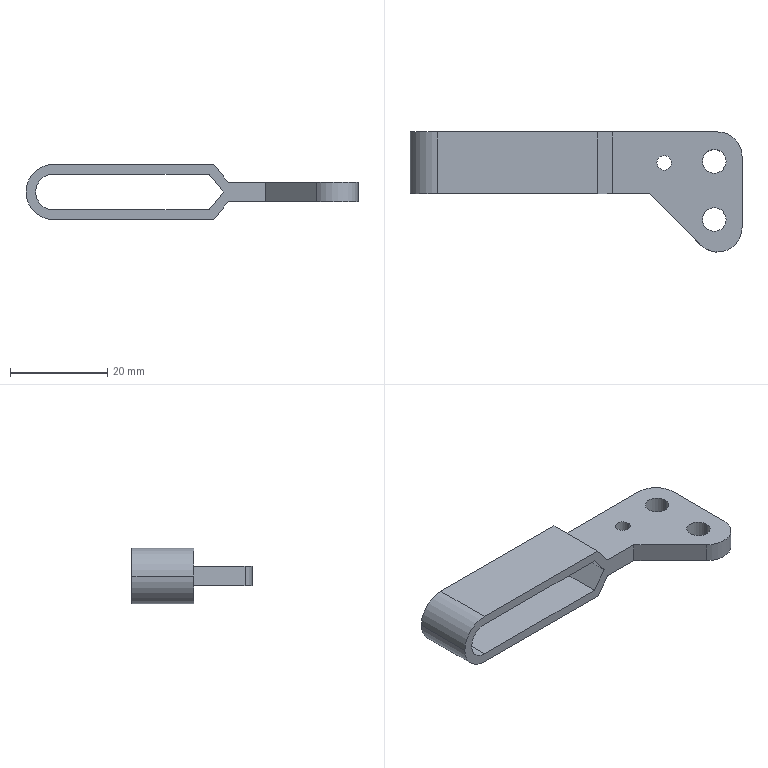Part | STEP file | 11-ARM_MC01-S311 | 1 solid | 25 faces | box 68.35 x 24.739 x 11.4 mm | volume 4057 mm3 | plane 14 | cylinder 11 | commonest cylinder face diameters 4.85 x4 3 x2 10 x2 11.4 x2 7.4 x1
STEP:
#1=CARTESIAN_POINT('',(-11.8,11.69,-4.));
#2=VERTEX_POINT('',#1);
#3=CARTESIAN_POINT('',(-8.8,11.69,-4.));
#4=VERTEX_POINT('',#3);
#5=CARTESIAN_POINT('',(-10.3,11.69,-4.));
#6=DIRECTION('',(0.,0.,1.));
#7=DIRECTION('',(1.,0.,0.));
#8=AXIS2_PLACEMENT_3D('',#5,#6,#7);
#9=CIRCLE('',#8,1.5);
#10=EDGE_CURVE('',#2,#4,#9,.T.);
#11=ORIENTED_EDGE('',*,*,#10,.F.);
#12=CARTESIAN_POINT('',(-11.8,11.69,0.));
#13=VERTEX_POINT('',#12);
#14=CARTESIAN_POINT('',(-11.8,11.69,0.));
#15=DIRECTION('',(0.,0.,1.));
#16=VECTOR('',#15,1000.);
#17=LINE('',#14,#16);
#18=EDGE_CURVE('',#2,#13,#17,.T.);
#19=ORIENTED_EDGE('',*,*,#18,.T.);
#20=CARTESIAN_POINT('',(-8.8,11.69,0.));
#21=VERTEX_POINT('',#20);
#22=CARTESIAN_POINT('',(-10.3,11.69,0.));
#23=DIRECTION('',(0.,0.,1.));
#24=DIRECTION('',(1.,0.,0.));
#25=AXIS2_PLACEMENT_3D('',#22,#23,#24);
#26=CIRCLE('',#25,1.5);
#27=EDGE_CURVE('',#13,#21,#26,.T.);
#28=ORIENTED_EDGE('',*,*,#27,.T.);
#29=CARTESIAN_POINT('',(-8.8,11.69,0.));
#30=DIRECTION('',(0.,0.,1.));
#31=VECTOR('',#30,1000.);
#32=LINE('',#29,#31);
#33=EDGE_CURVE('',#4,#21,#32,.T.);
#34=ORIENTED_EDGE('',*,*,#33,.F.);
#35=EDGE_LOOP('',(#11,#19,#28,#34));
#36=FACE_OUTER_BOUND('',#35,.T.);
#37=CARTESIAN_POINT('',(-10.3,11.69,0.));
#38=DIRECTION('',(0.,0.,1.));
#39=DIRECTION('',(1.,0.,0.));
#40=AXIS2_PLACEMENT_3D('',#37,#38,#39);
#41=CYLINDRICAL_SURFACE('',#40,1.5);
#42=ADVANCED_FACE('',(#36),#41,.F.);
#43=CARTESIAN_POINT('',(-2.425,12.,-4.));
#44=VERTEX_POINT('',#43);
#45=CARTESIAN_POINT('',(2.425,12.,-4.));
#46=VERTEX_POINT('',#45);
#47=CARTESIAN_POINT('',(0.,12.,-4.));
#48=DIRECTION('',(0.,0.,1.));
#49=DIRECTION('',(1.,0.,0.));
#50=AXIS2_PLACEMENT_3D('',#47,#48,#49);
#51=CIRCLE('',#50,2.425);
#52=EDGE_CURVE('',#44,#46,#51,.T.);
#53=ORIENTED_EDGE('',*,*,#52,.F.);
#54=CARTESIAN_POINT('',(-2.425,12.,0.));
#55=VERTEX_POINT('',#54);
#56=CARTESIAN_POINT('',(-2.425,12.,0.));
#57=DIRECTION('',(0.,0.,1.));
#58=VECTOR('',#57,1000.);
#59=LINE('',#56,#58);
#60=EDGE_CURVE('',#44,#55,#59,.T.);
#61=ORIENTED_EDGE('',*,*,#60,.T.);
#62=CARTESIAN_POINT('',(2.425,12.,0.));
#63=VERTEX_POINT('',#62);
#64=CARTESIAN_POINT('',(0.,12.,0.));
#65=DIRECTION('',(0.,0.,1.));
#66=DIRECTION('',(1.,0.,0.));
#67=AXIS2_PLACEMENT_3D('',#64,#65,#66);
#68=CIRCLE('',#67,2.425);
#69=EDGE_CURVE('',#55,#63,#68,.T.);
#70=ORIENTED_EDGE('',*,*,#69,.T.);
#71=CARTESIAN_POINT('',(2.425,12.,0.));
#72=DIRECTION('',(0.,0.,1.));
#73=VECTOR('',#72,1000.);
#74=LINE('',#71,#73);
#75=EDGE_CURVE('',#46,#63,#74,.T.);
#76=ORIENTED_EDGE('',*,*,#75,.F.);
#77=EDGE_LOOP('',(#53,#61,#70,#76));
#78=FACE_OUTER_BOUND('',#77,.T.);
#79=CARTESIAN_POINT('',(0.,12.,0.));
#80=DIRECTION('',(0.,0.,1.));
#81=DIRECTION('',(1.,0.,0.));
#82=AXIS2_PLACEMENT_3D('',#79,#80,#81);
#83=CYLINDRICAL_SURFACE('',#82,2.425);
#84=ADVANCED_FACE('',(#78),#83,.F.);
#85=CARTESIAN_POINT('',(-2.425,0.,-4.));
#86=VERTEX_POINT('',#85);
#87=CARTESIAN_POINT('',(2.425,0.,-4.));
#88=VERTEX_POINT('',#87);
#89=CARTESIAN_POINT('',(0.,0.,-4.));
#90=DIRECTION('',(0.,0.,1.));
#91=DIRECTION('',(1.,0.,0.));
#92=AXIS2_PLACEMENT_3D('',#89,#90,#91);
#93=CIRCLE('',#92,2.425);
#94=EDGE_CURVE('',#86,#88,#93,.T.);
#95=ORIENTED_EDGE('',*,*,#94,.F.);
#96=CARTESIAN_POINT('',(-2.425,0.,0.));
#97=VERTEX_POINT('',#96);
#98=CARTESIAN_POINT('',(-2.425,0.,0.));
#99=DIRECTION('',(0.,0.,1.));
#100=VECTOR('',#99,1000.);
#101=LINE('',#98,#100);
#102=EDGE_CURVE('',#86,#97,#101,.T.);
#103=ORIENTED_EDGE('',*,*,#102,.T.);
#104=CARTESIAN_POINT('',(2.425,0.,0.));
#105=VERTEX_POINT('',#104);
#106=CARTESIAN_POINT('',(0.,0.,0.));
#107=DIRECTION('',(0.,0.,1.));
#108=DIRECTION('',(1.,0.,0.));
#109=AXIS2_PLACEMENT_3D('',#106,#107,#108);
#110=CIRCLE('',#109,2.425);
#111=EDGE_CURVE('',#97,#105,#110,.T.);
#112=ORIENTED_EDGE('',*,*,#111,.T.);
#113=CARTESIAN_POINT('',(2.425,0.,0.));
#114=DIRECTION('',(0.,0.,1.));
#115=VECTOR('',#114,1000.);
#116=LINE('',#113,#115);
#117=EDGE_CURVE('',#88,#105,#116,.T.);
#118=ORIENTED_EDGE('',*,*,#117,.F.);
#119=EDGE_LOOP('',(#95,#103,#112,#118));
#120=FACE_OUTER_BOUND('',#119,.T.);
#121=CARTESIAN_POINT('',(0.,0.,0.));
#122=DIRECTION('',(0.,0.,1.));
#123=DIRECTION('',(1.,0.,0.));
#124=AXIS2_PLACEMENT_3D('',#121,#122,#123);
#125=CYLINDRICAL_SURFACE('',#124,2.425);
#126=ADVANCED_FACE('',(#120),#125,.F.);
#127=CARTESIAN_POINT('',(-21.998,18.05,-2.));
#128=VERTEX_POINT('',#127);
#129=CARTESIAN_POINT('',(-24.95,18.05,-5.7));
#130=VERTEX_POINT('',#129);
#131=CARTESIAN_POINT('',(-24.95,18.05,-5.7));
#132=DIRECTION('',(-0.6237,0.,-0.7817));
#133=VECTOR('',#132,1000.);
#134=LINE('',#131,#133);
#135=EDGE_CURVE('',#128,#130,#134,.T.);
#136=ORIENTED_EDGE('',*,*,#135,.F.);
#137=CARTESIAN_POINT('',(-24.95,18.05,1.7));
#138=VERTEX_POINT('',#137);
#139=CARTESIAN_POINT('',(-24.95,18.05,1.7));
#140=DIRECTION('',(0.6237,0.,-0.7817));
#141=VECTOR('',#140,1000.);
#142=LINE('',#139,#141);
#143=EDGE_CURVE('',#138,#128,#142,.T.);
#144=ORIENTED_EDGE('',*,*,#143,.F.);
#145=CARTESIAN_POINT('',(-56.95,18.05,1.7));
#146=VERTEX_POINT('',#145);
#147=CARTESIAN_POINT('',(-56.95,18.05,1.7));
#148=DIRECTION('',(1.,0.,0.));
#149=VECTOR('',#148,1000.);
#150=LINE('',#147,#149);
#151=EDGE_CURVE('',#146,#138,#150,.T.);
#152=ORIENTED_EDGE('',*,*,#151,.F.);
#153=CARTESIAN_POINT('',(-56.95,18.05,-5.7));
#154=VERTEX_POINT('',#153);
#155=CARTESIAN_POINT('',(-56.95,18.05,-2.));
#156=DIRECTION('',(0.,1.,0.));
#157=DIRECTION('',(0.,0.,1.));
#158=AXIS2_PLACEMENT_3D('',#155,#156,#157);
#159=CIRCLE('',#158,3.7);
#160=EDGE_CURVE('',#154,#146,#159,.T.);
#161=ORIENTED_EDGE('',*,*,#160,.F.);
#162=CARTESIAN_POINT('',(-24.95,18.05,-5.7));
#163=DIRECTION('',(-1.,0.,0.));
#164=VECTOR('',#163,1000.);
#165=LINE('',#162,#164);
#166=EDGE_CURVE('',#130,#154,#165,.T.);
#167=ORIENTED_EDGE('',*,*,#166,.F.);
#168=EDGE_LOOP('',(#136,#144,#152,#161,#167));
#169=FACE_BOUND('',#168,.T.);
#170=CARTESIAN_POINT('',(0.7,18.05,0.));
#171=VERTEX_POINT('',#170);
#172=CARTESIAN_POINT('',(-21.035,18.05,0.));
#173=VERTEX_POINT('',#172);
#174=CARTESIAN_POINT('',(-21.035,18.05,0.));
#175=DIRECTION('',(-1.,0.,0.));
#176=VECTOR('',#175,1000.);
#177=LINE('',#174,#176);
#178=EDGE_CURVE('',#171,#173,#177,.T.);
#179=ORIENTED_EDGE('',*,*,#178,.F.);
#180=CARTESIAN_POINT('',(0.7,18.05,-4.));
#181=VERTEX_POINT('',#180);
#182=CARTESIAN_POINT('',(0.7,18.05,3.7));
#183=DIRECTION('',(0.,0.,-1.));
#184=VECTOR('',#183,1000.);
#185=LINE('',#182,#184);
#186=EDGE_CURVE('',#171,#181,#185,.T.);
#187=ORIENTED_EDGE('',*,*,#186,.T.);
#188=CARTESIAN_POINT('',(-21.035,18.05,-4.));
#189=VERTEX_POINT('',#188);
#190=CARTESIAN_POINT('',(-21.035,18.05,-4.));
#191=DIRECTION('',(1.,0.,0.));
#192=VECTOR('',#191,1000.);
#193=LINE('',#190,#192);
#194=EDGE_CURVE('',#189,#181,#193,.T.);
#195=ORIENTED_EDGE('',*,*,#194,.F.);
#196=CARTESIAN_POINT('',(-23.987,18.05,-7.7));
#197=VERTEX_POINT('',#196);
#198=CARTESIAN_POINT('',(-23.987,18.05,-7.7));
#199=DIRECTION('',(0.6237,0.,0.7817));
#200=VECTOR('',#199,1000.);
#201=LINE('',#198,#200);
#202=EDGE_CURVE('',#197,#189,#201,.T.);
#203=ORIENTED_EDGE('',*,*,#202,.F.);
#204=CARTESIAN_POINT('',(-56.95,18.05,-7.7));
#205=VERTEX_POINT('',#204);
#206=CARTESIAN_POINT('',(-62.65,18.05,-7.7));
#207=DIRECTION('',(-1.,0.,0.));
#208=VECTOR('',#207,1000.);
#209=LINE('',#206,#208);
#210=EDGE_CURVE('',#197,#205,#209,.T.);
#211=ORIENTED_EDGE('',*,*,#210,.T.);
#212=CARTESIAN_POINT('',(-62.65,18.05,-2.));
#213=VERTEX_POINT('',#212);
#214=CARTESIAN_POINT('',(-56.95,18.05,-2.));
#215=DIRECTION('',(0.,1.,0.));
#216=DIRECTION('',(0.,0.,-1.));
#217=AXIS2_PLACEMENT_3D('',#214,#215,#216);
#218=CIRCLE('',#217,5.7);
#219=EDGE_CURVE('',#205,#213,#218,.T.);
#220=ORIENTED_EDGE('',*,*,#219,.T.);
#221=CARTESIAN_POINT('',(-56.95,18.05,3.7));
#222=VERTEX_POINT('',#221);
#223=CARTESIAN_POINT('',(-56.95,18.05,-2.));
#224=DIRECTION('',(0.,1.,0.));
#225=DIRECTION('',(0.,0.,-1.));
#226=AXIS2_PLACEMENT_3D('',#223,#224,#225);
#227=CIRCLE('',#226,5.7);
#228=EDGE_CURVE('',#213,#222,#227,.T.);
#229=ORIENTED_EDGE('',*,*,#228,.T.);
#230=CARTESIAN_POINT('',(-23.987,18.05,3.7));
#231=VERTEX_POINT('',#230);
#232=CARTESIAN_POINT('',(-62.65,18.05,3.7));
#233=DIRECTION('',(-1.,0.,0.));
#234=VECTOR('',#233,1000.);
#235=LINE('',#232,#234);
#236=EDGE_CURVE('',#231,#222,#235,.T.);
#237=ORIENTED_EDGE('',*,*,#236,.F.);
#238=CARTESIAN_POINT('',(-23.987,18.05,3.7));
#239=DIRECTION('',(-0.6237,0.,0.7817));
#240=VECTOR('',#239,1000.);
#241=LINE('',#238,#240);
#242=EDGE_CURVE('',#173,#231,#241,.T.);
#243=ORIENTED_EDGE('',*,*,#242,.F.);
#244=EDGE_LOOP('',(#179,#187,#195,#203,#211,#220,#229,#237,#243));
#245=FACE_OUTER_BOUND('',#244,.T.);
#246=CARTESIAN_POINT('',(-62.65,18.05,3.7));
#247=DIRECTION('',(0.,-1.,0.));
#248=DIRECTION('',(0.,0.,-1.));
#249=AXIS2_PLACEMENT_3D('',#246,#247,#248);
#250=PLANE('',#249);
#251=ADVANCED_FACE('',(#169,#245),#250,.F.);
#252=CARTESIAN_POINT('',(-56.95,5.35,1.7));
#253=VERTEX_POINT('',#252);
#254=CARTESIAN_POINT('',(-24.95,5.35,1.7));
#255=VERTEX_POINT('',#254);
#256=CARTESIAN_POINT('',(-62.65,5.35,1.7));
#257=DIRECTION('',(1.,0.,0.));
#258=VECTOR('',#257,1000.);
#259=LINE('',#256,#258);
#260=EDGE_CURVE('',#253,#255,#259,.T.);
#261=ORIENTED_EDGE('',*,*,#260,.T.);
#262=CARTESIAN_POINT('',(-21.998,5.35,-2.));
#263=VERTEX_POINT('',#262);
#264=CARTESIAN_POINT('',(-40.59,5.35,21.302));
#265=DIRECTION('',(0.6237,0.,-0.7817));
#266=VECTOR('',#265,1000.);
#267=LINE('',#264,#266);
#268=EDGE_CURVE('',#255,#263,#267,.T.);
#269=ORIENTED_EDGE('',*,*,#268,.T.);
#270=CARTESIAN_POINT('',(-24.95,5.35,-5.7));
#271=VERTEX_POINT('',#270);
#272=CARTESIAN_POINT('',(-35.032,5.35,-18.336));
#273=DIRECTION('',(-0.6237,0.,-0.7817));
#274=VECTOR('',#273,1000.);
#275=LINE('',#272,#274);
#276=EDGE_CURVE('',#263,#271,#275,.T.);
#277=ORIENTED_EDGE('',*,*,#276,.T.);
#278=CARTESIAN_POINT('',(-56.95,5.35,-5.7));
#279=VERTEX_POINT('',#278);
#280=CARTESIAN_POINT('',(-62.65,5.35,-5.7));
#281=DIRECTION('',(-1.,0.,0.));
#282=VECTOR('',#281,1000.);
#283=LINE('',#280,#282);
#284=EDGE_CURVE('',#271,#279,#283,.T.);
#285=ORIENTED_EDGE('',*,*,#284,.T.);
#286=CARTESIAN_POINT('',(-56.95,5.35,-2.));
#287=DIRECTION('',(0.,1.,0.));
#288=DIRECTION('',(-1.,0.,0.));
#289=AXIS2_PLACEMENT_3D('',#286,#287,#288);
#290=CIRCLE('',#289,3.7);
#291=EDGE_CURVE('',#279,#253,#290,.T.);
#292=ORIENTED_EDGE('',*,*,#291,.T.);
#293=EDGE_LOOP('',(#261,#269,#277,#285,#292));
#294=FACE_BOUND('',#293,.T.);
#295=CARTESIAN_POINT('',(-56.95,5.35,-7.7));
#296=VERTEX_POINT('',#295);
#297=CARTESIAN_POINT('',(-23.987,5.35,-7.7));
#298=VERTEX_POINT('',#297);
#299=CARTESIAN_POINT('',(-62.65,5.35,-7.7));
#300=DIRECTION('',(1.,0.,0.));
#301=VECTOR('',#300,1000.);
#302=LINE('',#299,#301);
#303=EDGE_CURVE('',#296,#298,#302,.T.);
#304=ORIENTED_EDGE('',*,*,#303,.T.);
#305=CARTESIAN_POINT('',(-21.035,5.35,-4.));
#306=VERTEX_POINT('',#305);
#307=CARTESIAN_POINT('',(-33.469,5.35,-19.583));
#308=DIRECTION('',(0.6237,0.,0.7817));
#309=VECTOR('',#308,1000.);
#310=LINE('',#307,#309);
#311=EDGE_CURVE('',#298,#306,#310,.T.);
#312=ORIENTED_EDGE('',*,*,#311,.T.);
#313=CARTESIAN_POINT('',(-13.41,5.35,-4.));
#314=VERTEX_POINT('',#313);
#315=CARTESIAN_POINT('',(-62.65,5.35,-4.));
#316=DIRECTION('',(1.,0.,0.));
#317=VECTOR('',#316,1000.);
#318=LINE('',#315,#317);
#319=EDGE_CURVE('',#306,#314,#318,.T.);
#320=ORIENTED_EDGE('',*,*,#319,.T.);
#321=CARTESIAN_POINT('',(-13.41,5.35,0.));
#322=VERTEX_POINT('',#321);
#323=CARTESIAN_POINT('',(-13.41,5.35,3.7));
#324=DIRECTION('',(0.,0.,-1.));
#325=VECTOR('',#324,1000.);
#326=LINE('',#323,#325);
#327=EDGE_CURVE('',#322,#314,#326,.T.);
#328=ORIENTED_EDGE('',*,*,#327,.F.);
#329=CARTESIAN_POINT('',(-21.035,5.35,0.));
#330=VERTEX_POINT('',#329);
#331=CARTESIAN_POINT('',(-62.65,5.35,0.));
#332=DIRECTION('',(-1.,0.,0.));
#333=VECTOR('',#332,1000.);
#334=LINE('',#331,#333);
#335=EDGE_CURVE('',#322,#330,#334,.T.);
#336=ORIENTED_EDGE('',*,*,#335,.T.);
#337=CARTESIAN_POINT('',(-23.987,5.35,3.7));
#338=VERTEX_POINT('',#337);
#339=CARTESIAN_POINT('',(-39.026,5.35,22.549));
#340=DIRECTION('',(-0.6237,0.,0.7817));
#341=VECTOR('',#340,1000.);
#342=LINE('',#339,#341);
#343=EDGE_CURVE('',#330,#338,#342,.T.);
#344=ORIENTED_EDGE('',*,*,#343,.T.);
#345=CARTESIAN_POINT('',(-56.95,5.35,3.7));
#346=VERTEX_POINT('',#345);
#347=CARTESIAN_POINT('',(-62.65,5.35,3.7));
#348=DIRECTION('',(1.,0.,0.));
#349=VECTOR('',#348,1000.);
#350=LINE('',#347,#349);
#351=EDGE_CURVE('',#346,#338,#350,.T.);
#352=ORIENTED_EDGE('',*,*,#351,.F.);
#353=CARTESIAN_POINT('',(-62.65,5.35,-2.));
#354=VERTEX_POINT('',#353);
#355=CARTESIAN_POINT('',(-56.95,5.35,-2.));
#356=DIRECTION('',(0.,-1.,0.));
#357=DIRECTION('',(-1.,0.,0.));
#358=AXIS2_PLACEMENT_3D('',#355,#356,#357);
#359=CIRCLE('',#358,5.7);
#360=EDGE_CURVE('',#346,#354,#359,.T.);
#361=ORIENTED_EDGE('',*,*,#360,.T.);
#362=CARTESIAN_POINT('',(-56.95,5.35,-2.));
#363=DIRECTION('',(0.,-1.,0.));
#364=DIRECTION('',(-1.,0.,0.));
#365=AXIS2_PLACEMENT_3D('',#362,#363,#364);
#366=CIRCLE('',#365,5.7);
#367=EDGE_CURVE('',#354,#296,#366,.T.);
#368=ORIENTED_EDGE('',*,*,#367,.T.);
#369=EDGE_LOOP('',(#304,#312,#320,#328,#336,#344,#352,#361,#368));
#370=FACE_OUTER_BOUND('',#369,.T.);
#371=CARTESIAN_POINT('',(-62.65,5.35,3.7));
#372=DIRECTION('',(0.,1.,0.));
#373=DIRECTION('',(-1.,0.,0.));
#374=AXIS2_PLACEMENT_3D('',#371,#372,#373);
#375=PLANE('',#374);
#376=ADVANCED_FACE('',(#294,#370),#375,.F.);
#377=ORIENTED_EDGE('',*,*,#327,.T.);
#378=CARTESIAN_POINT('',(-2.836,-5.224,-4.));
#379=VERTEX_POINT('',#378);
#380=CARTESIAN_POINT('',(-13.41,5.35,-4.));
#381=DIRECTION('',(0.7071,-0.7071,0.));
#382=VECTOR('',#381,1000.);
#383=LINE('',#380,#382);
#384=EDGE_CURVE('',#314,#379,#383,.T.);
#385=ORIENTED_EDGE('',*,*,#384,.T.);
#386=CARTESIAN_POINT('',(-2.836,-5.224,0.));
#387=VERTEX_POINT('',#386);
#388=CARTESIAN_POINT('',(-2.836,-5.224,3.7));
#389=DIRECTION('',(0.,0.,-1.));
#390=VECTOR('',#389,1000.);
#391=LINE('',#388,#390);
#392=EDGE_CURVE('',#387,#379,#391,.T.);
#393=ORIENTED_EDGE('',*,*,#392,.F.);
#394=CARTESIAN_POINT('',(-13.41,5.35,0.));
#395=DIRECTION('',(-0.7071,0.7071,0.));
#396=VECTOR('',#395,1000.);
#397=LINE('',#394,#396);
#398=EDGE_CURVE('',#387,#322,#397,.T.);
#399=ORIENTED_EDGE('',*,*,#398,.T.);
#400=EDGE_LOOP('',(#377,#385,#393,#399));
#401=FACE_OUTER_BOUND('',#400,.T.);
#402=CARTESIAN_POINT('',(-13.41,5.35,3.7));
#403=DIRECTION('',(0.7071,0.7071,0.));
#404=DIRECTION('',(-0.7071,0.7071,0.));
#405=AXIS2_PLACEMENT_3D('',#402,#403,#404);
#406=PLANE('',#405);
#407=ADVANCED_FACE('',(#401),#406,.F.);
#408=ORIENTED_EDGE('',*,*,#392,.T.);
#409=CARTESIAN_POINT('',(5.7,-1.689,-4.));
#410=VERTEX_POINT('',#409);
#411=CARTESIAN_POINT('',(0.7,-1.689,-4.));
#412=DIRECTION('',(0.,0.,1.));
#413=DIRECTION('',(1.,0.,0.));
#414=AXIS2_PLACEMENT_3D('',#411,#412,#413);
#415=CIRCLE('',#414,5.);
#416=EDGE_CURVE('',#379,#410,#415,.T.);
#417=ORIENTED_EDGE('',*,*,#416,.T.);
#418=CARTESIAN_POINT('',(5.7,-1.689,0.));
#419=VERTEX_POINT('',#418);
#420=CARTESIAN_POINT('',(5.7,-1.689,3.7));
#421=DIRECTION('',(0.,0.,-1.));
#422=VECTOR('',#421,1000.);
#423=LINE('',#420,#422);
#424=EDGE_CURVE('',#419,#410,#423,.T.);
#425=ORIENTED_EDGE('',*,*,#424,.F.);
#426=CARTESIAN_POINT('',(0.7,-1.689,0.));
#427=DIRECTION('',(0.,0.,-1.));
#428=DIRECTION('',(-1.,0.,0.));
#429=AXIS2_PLACEMENT_3D('',#426,#427,#428);
#430=CIRCLE('',#429,5.);
#431=EDGE_CURVE('',#419,#387,#430,.T.);
#432=ORIENTED_EDGE('',*,*,#431,.T.);
#433=EDGE_LOOP('',(#408,#417,#425,#432));
#434=FACE_OUTER_BOUND('',#433,.T.);
#435=CARTESIAN_POINT('',(0.7,-1.689,3.7));
#436=DIRECTION('',(0.,0.,-1.));
#437=DIRECTION('',(-1.,0.,0.));
#438=AXIS2_PLACEMENT_3D('',#435,#436,#437);
#439=CYLINDRICAL_SURFACE('',#438,5.);
#440=ADVANCED_FACE('',(#434),#439,.T.);
#441=CARTESIAN_POINT('',(5.7,13.05,-4.));
#442=VERTEX_POINT('',#441);
#443=CARTESIAN_POINT('',(5.7,-6.689,-4.));
#444=DIRECTION('',(0.,1.,0.));
#445=VECTOR('',#444,1000.);
#446=LINE('',#443,#445);
#447=EDGE_CURVE('',#410,#442,#446,.T.);
#448=ORIENTED_EDGE('',*,*,#447,.T.);
#449=CARTESIAN_POINT('',(5.7,13.05,0.));
#450=VERTEX_POINT('',#449);
#451=CARTESIAN_POINT('',(5.7,13.05,3.7));
#452=DIRECTION('',(0.,0.,1.));
#453=VECTOR('',#452,1000.);
#454=LINE('',#451,#453);
#455=EDGE_CURVE('',#442,#450,#454,.T.);
#456=ORIENTED_EDGE('',*,*,#455,.T.);
#457=CARTESIAN_POINT('',(5.7,-6.689,0.));
#458=DIRECTION('',(0.,1.,0.));
#459=VECTOR('',#458,1000.);
#460=LINE('',#457,#459);
#461=EDGE_CURVE('',#419,#450,#460,.T.);
#462=ORIENTED_EDGE('',*,*,#461,.F.);
#463=ORIENTED_EDGE('',*,*,#424,.T.);
#464=EDGE_LOOP('',(#448,#456,#462,#463));
#465=FACE_OUTER_BOUND('',#464,.T.);
#466=CARTESIAN_POINT('',(5.7,-1.689,3.7));
#467=DIRECTION('',(-1.,0.,0.));
#468=DIRECTION('',(0.,-1.,0.));
#469=AXIS2_PLACEMENT_3D('',#466,#467,#468);
#470=PLANE('',#469);
#471=ADVANCED_FACE('',(#465),#470,.F.);
#472=CARTESIAN_POINT('',(-23.987,-1.689,3.7));
#473=DIRECTION('',(0.,-1.,0.));
#474=VECTOR('',#473,1000.);
#475=LINE('',#472,#474);
#476=EDGE_CURVE('',#231,#338,#475,.T.);
#477=ORIENTED_EDGE('',*,*,#476,.F.);
#478=ORIENTED_EDGE('',*,*,#236,.T.);
#479=CARTESIAN_POINT('',(-56.95,5.35,3.7));
#480=DIRECTION('',(0.,-1.,0.));
#481=VECTOR('',#480,1000.);
#482=LINE('',#479,#481);
#483=EDGE_CURVE('',#222,#346,#482,.T.);
#484=ORIENTED_EDGE('',*,*,#483,.T.);
#485=ORIENTED_EDGE('',*,*,#351,.T.);
#486=EDGE_LOOP('',(#477,#478,#484,#485));
#487=FACE_OUTER_BOUND('',#486,.T.);
#488=CARTESIAN_POINT('',(0.7,-1.689,3.7));
#489=DIRECTION('',(0.,0.,1.));
#490=DIRECTION('',(1.,0.,0.));
#491=AXIS2_PLACEMENT_3D('',#488,#489,#490);
#492=PLANE('',#491);
#493=ADVANCED_FACE('',(#487),#492,.T.);
#494=ORIENTED_EDGE('',*,*,#210,.F.);
#495=CARTESIAN_POINT('',(-23.987,-1.689,-7.7));
#496=DIRECTION('',(0.,-1.,0.));
#497=VECTOR('',#496,1000.);
#498=LINE('',#495,#497);
#499=EDGE_CURVE('',#197,#298,#498,.T.);
#500=ORIENTED_EDGE('',*,*,#499,.T.);
#501=ORIENTED_EDGE('',*,*,#303,.F.);
#502=CARTESIAN_POINT('',(-56.95,-1.689,-7.7));
#503=DIRECTION('',(0.,1.,0.));
#504=VECTOR('',#503,1000.);
#505=LINE('',#502,#504);
#506=EDGE_CURVE('',#296,#205,#505,.T.);
#507=ORIENTED_EDGE('',*,*,#506,.T.);
#508=EDGE_LOOP('',(#494,#500,#501,#507));
#509=FACE_OUTER_BOUND('',#508,.T.);
#510=CARTESIAN_POINT('',(0.7,-1.689,-7.7));
#511=DIRECTION('',(0.,0.,1.));
#512=DIRECTION('',(1.,0.,0.));
#513=AXIS2_PLACEMENT_3D('',#510,#511,#512);
#514=PLANE('',#513);
#515=ADVANCED_FACE('',(#509),#514,.F.);
#516=ORIENTED_EDGE('',*,*,#483,.F.);
#517=ORIENTED_EDGE('',*,*,#228,.F.);
#518=CARTESIAN_POINT('',(-62.65,18.05,-2.));
#519=DIRECTION('',(0.,1.,0.));
#520=VECTOR('',#519,1000.);
#521=LINE('',#518,#520);
#522=EDGE_CURVE('',#354,#213,#521,.T.);
#523=ORIENTED_EDGE('',*,*,#522,.F.);
#524=ORIENTED_EDGE('',*,*,#360,.F.);
#525=EDGE_LOOP('',(#516,#517,#523,#524));
#526=FACE_OUTER_BOUND('',#525,.T.);
#527=CARTESIAN_POINT('',(-56.95,-1.689,-2.));
#528=DIRECTION('',(0.,1.,0.));
#529=DIRECTION('',(0.,0.,1.));
#530=AXIS2_PLACEMENT_3D('',#527,#528,#529);
#531=CYLINDRICAL_SURFACE('',#530,5.7);
#532=ADVANCED_FACE('',(#526),#531,.T.);
#533=ORIENTED_EDGE('',*,*,#219,.F.);
#534=ORIENTED_EDGE('',*,*,#506,.F.);
#535=ORIENTED_EDGE('',*,*,#367,.F.);
#536=ORIENTED_EDGE('',*,*,#522,.T.);
#537=EDGE_LOOP('',(#533,#534,#535,#536));
#538=FACE_OUTER_BOUND('',#537,.T.);
#539=CARTESIAN_POINT('',(-56.95,18.05,-2.));
#540=DIRECTION('',(0.,-1.,0.));
#541=DIRECTION('',(0.,0.,-1.));
#542=AXIS2_PLACEMENT_3D('',#539,#540,#541);
#543=CYLINDRICAL_SURFACE('',#542,5.7);
#544=ADVANCED_FACE('',(#538),#543,.T.);
#545=CARTESIAN_POINT('',(-10.3,11.69,0.));
#546=DIRECTION('',(0.,0.,1.));
#547=DIRECTION('',(1.,0.,0.));
#548=AXIS2_PLACEMENT_3D('',#545,#546,#547);
#549=CIRCLE('',#548,1.5);
#550=EDGE_CURVE('',#21,#13,#549,.T.);
#551=ORIENTED_EDGE('',*,*,#550,.F.);
#552=ORIENTED_EDGE('',*,*,#27,.F.);
#553=EDGE_LOOP('',(#551,#552));
#554=FACE_BOUND('',#553,.T.);
#555=CARTESIAN_POINT('',(0.,12.,0.));
#556=DIRECTION('',(0.,0.,1.));
#557=DIRECTION('',(1.,0.,0.));
#558=AXIS2_PLACEMENT_3D('',#555,#556,#557);
#559=CIRCLE('',#558,2.425);
#560=EDGE_CURVE('',#63,#55,#559,.T.);
#561=ORIENTED_EDGE('',*,*,#560,.F.);
#562=ORIENTED_EDGE('',*,*,#69,.F.);
#563=EDGE_LOOP('',(#561,#562));
#564=FACE_BOUND('',#563,.T.);
#565=CARTESIAN_POINT('',(0.,0.,0.));
#566=DIRECTION('',(0.,0.,1.));
#567=DIRECTION('',(1.,0.,0.));
#568=AXIS2_PLACEMENT_3D('',#565,#566,#567);
#569=CIRCLE('',#568,2.425);
#570=EDGE_CURVE('',#105,#97,#569,.T.);
#571=ORIENTED_EDGE('',*,*,#570,.F.);
#572=ORIENTED_EDGE('',*,*,#111,.F.);
#573=EDGE_LOOP('',(#571,#572));
#574=FACE_BOUND('',#573,.T.);
#575=ORIENTED_EDGE('',*,*,#461,.T.);
#576=CARTESIAN_POINT('',(0.7,13.05,0.));
#577=DIRECTION('',(0.,0.,1.));
#578=DIRECTION('',(-1.,0.,0.));
#579=AXIS2_PLACEMENT_3D('',#576,#577,#578);
#580=CIRCLE('',#579,5.);
#581=EDGE_CURVE('',#450,#171,#580,.T.);
#582=ORIENTED_EDGE('',*,*,#581,.T.);
#583=ORIENTED_EDGE('',*,*,#178,.T.);
#584=CARTESIAN_POINT('',(-21.035,-6.689,0.));
#585=DIRECTION('',(0.,1.,0.));
#586=VECTOR('',#585,1000.);
#587=LINE('',#584,#586);
#588=EDGE_CURVE('',#330,#173,#587,.T.);
#589=ORIENTED_EDGE('',*,*,#588,.F.);
#590=ORIENTED_EDGE('',*,*,#335,.F.);
#591=ORIENTED_EDGE('',*,*,#398,.F.);
#592=ORIENTED_EDGE('',*,*,#431,.F.);
#593=EDGE_LOOP('',(#575,#582,#583,#589,#590,#591,#592));
#594=FACE_OUTER_BOUND('',#593,.T.);
#595=CARTESIAN_POINT('',(-21.035,-6.689,0.));
#596=DIRECTION('',(0.,0.,-1.));
#597=DIRECTION('',(-1.,0.,0.));
#598=AXIS2_PLACEMENT_3D('',#595,#596,#597);
#599=PLANE('',#598);
#600=ADVANCED_FACE('',(#554,#564,#574,#594),#599,.F.);
#601=ORIENTED_EDGE('',*,*,#588,.T.);
#602=ORIENTED_EDGE('',*,*,#242,.T.);
#603=ORIENTED_EDGE('',*,*,#476,.T.);
#604=ORIENTED_EDGE('',*,*,#343,.F.);
#605=EDGE_LOOP('',(#601,#602,#603,#604));
#606=FACE_OUTER_BOUND('',#605,.T.);
#607=CARTESIAN_POINT('',(-23.987,-6.689,3.7));
#608=DIRECTION('',(-0.7817,0.,-0.6237));
#609=DIRECTION('',(-0.6237,0.,0.7817));
#610=AXIS2_PLACEMENT_3D('',#607,#608,#609);
#611=PLANE('',#610);
#612=ADVANCED_FACE('',(#606),#611,.F.);
#613=CARTESIAN_POINT('',(-24.95,-6.689,1.7));
#614=DIRECTION('',(0.,1.,0.));
#615=VECTOR('',#614,1000.);
#616=LINE('',#613,#615);
#617=EDGE_CURVE('',#255,#138,#616,.T.);
#618=ORIENTED_EDGE('',*,*,#617,.T.);
#619=ORIENTED_EDGE('',*,*,#143,.T.);
#620=CARTESIAN_POINT('',(-21.998,-6.689,-2.));
#621=DIRECTION('',(0.,1.,0.));
#622=VECTOR('',#621,1000.);
#623=LINE('',#620,#622);
#624=EDGE_CURVE('',#263,#128,#623,.T.);
#625=ORIENTED_EDGE('',*,*,#624,.F.);
#626=ORIENTED_EDGE('',*,*,#268,.F.);
#627=EDGE_LOOP('',(#618,#619,#625,#626));
#628=FACE_OUTER_BOUND('',#627,.T.);
#629=CARTESIAN_POINT('',(-24.95,-6.689,1.7));
#630=DIRECTION('',(0.7817,0.,0.6237));
#631=DIRECTION('',(0.6237,0.,-0.7817));
#632=AXIS2_PLACEMENT_3D('',#629,#630,#631);
#633=PLANE('',#632);
#634=ADVANCED_FACE('',(#628),#633,.F.);
#635=CARTESIAN_POINT('',(-56.95,-6.689,1.7));
#636=DIRECTION('',(0.,1.,0.));
#637=VECTOR('',#636,1000.);
#638=LINE('',#635,#637);
#639=EDGE_CURVE('',#253,#146,#638,.T.);
#640=ORIENTED_EDGE('',*,*,#639,.T.);
#641=ORIENTED_EDGE('',*,*,#151,.T.);
#642=ORIENTED_EDGE('',*,*,#617,.F.);
#643=ORIENTED_EDGE('',*,*,#260,.F.);
#644=EDGE_LOOP('',(#640,#641,#642,#643));
#645=FACE_OUTER_BOUND('',#644,.T.);
#646=CARTESIAN_POINT('',(-56.95,-6.689,1.7));
#647=DIRECTION('',(0.,0.,1.));
#648=DIRECTION('',(1.,0.,0.));
#649=AXIS2_PLACEMENT_3D('',#646,#647,#648);
#650=PLANE('',#649);
#651=ADVANCED_FACE('',(#645),#650,.F.);
#652=CARTESIAN_POINT('',(-56.95,-6.689,-5.7));
#653=DIRECTION('',(0.,1.,0.));
#654=VECTOR('',#653,1000.);
#655=LINE('',#652,#654);
#656=EDGE_CURVE('',#279,#154,#655,.T.);
#657=ORIENTED_EDGE('',*,*,#656,.T.);
#658=ORIENTED_EDGE('',*,*,#160,.T.);
#659=ORIENTED_EDGE('',*,*,#639,.F.);
#660=ORIENTED_EDGE('',*,*,#291,.F.);
#661=EDGE_LOOP('',(#657,#658,#659,#660));
#662=FACE_OUTER_BOUND('',#661,.T.);
#663=CARTESIAN_POINT('',(-56.95,-6.689,-2.));
#664=DIRECTION('',(0.,1.,0.));
#665=DIRECTION('',(0.,0.,1.));
#666=AXIS2_PLACEMENT_3D('',#663,#664,#665);
#667=CYLINDRICAL_SURFACE('',#666,3.7);
#668=ADVANCED_FACE('',(#662),#667,.F.);
#669=CARTESIAN_POINT('',(-24.95,-6.689,-5.7));
#670=DIRECTION('',(0.,1.,0.));
#671=VECTOR('',#670,1000.);
#672=LINE('',#669,#671);
#673=EDGE_CURVE('',#271,#130,#672,.T.);
#674=ORIENTED_EDGE('',*,*,#673,.T.);
#675=ORIENTED_EDGE('',*,*,#166,.T.);
#676=ORIENTED_EDGE('',*,*,#656,.F.);
#677=ORIENTED_EDGE('',*,*,#284,.F.);
#678=EDGE_LOOP('',(#674,#675,#676,#677));
#679=FACE_OUTER_BOUND('',#678,.T.);
#680=CARTESIAN_POINT('',(-24.95,-6.689,-5.7));
#681=DIRECTION('',(0.,0.,-1.));
#682=DIRECTION('',(-1.,0.,0.));
#683=AXIS2_PLACEMENT_3D('',#680,#681,#682);
#684=PLANE('',#683);
#685=ADVANCED_FACE('',(#679),#684,.F.);
#686=ORIENTED_EDGE('',*,*,#624,.T.);
#687=ORIENTED_EDGE('',*,*,#135,.T.);
#688=ORIENTED_EDGE('',*,*,#673,.F.);
#689=ORIENTED_EDGE('',*,*,#276,.F.);
#690=EDGE_LOOP('',(#686,#687,#688,#689));
#691=FACE_OUTER_BOUND('',#690,.T.);
#692=CARTESIAN_POINT('',(-24.95,-6.689,-5.7));
#693=DIRECTION('',(0.7817,0.,-0.6237));
#694=DIRECTION('',(-0.6237,0.,-0.7817));
#695=AXIS2_PLACEMENT_3D('',#692,#693,#694);
#696=PLANE('',#695);
#697=ADVANCED_FACE('',(#691),#696,.F.);
#698=CARTESIAN_POINT('',(-10.3,11.69,-4.));
#699=DIRECTION('',(0.,0.,1.));
#700=DIRECTION('',(1.,0.,0.));
#701=AXIS2_PLACEMENT_3D('',#698,#699,#700);
#702=CIRCLE('',#701,1.5);
#703=EDGE_CURVE('',#4,#2,#702,.T.);
#704=ORIENTED_EDGE('',*,*,#703,.T.);
#705=ORIENTED_EDGE('',*,*,#10,.T.);
#706=EDGE_LOOP('',(#704,#705));
#707=FACE_BOUND('',#706,.T.);
#708=CARTESIAN_POINT('',(0.,12.,-4.));
#709=DIRECTION('',(0.,0.,1.));
#710=DIRECTION('',(1.,0.,0.));
#711=AXIS2_PLACEMENT_3D('',#708,#709,#710);
#712=CIRCLE('',#711,2.425);
#713=EDGE_CURVE('',#46,#44,#712,.T.);
#714=ORIENTED_EDGE('',*,*,#713,.T.);
#715=ORIENTED_EDGE('',*,*,#52,.T.);
#716=EDGE_LOOP('',(#714,#715));
#717=FACE_BOUND('',#716,.T.);
#718=CARTESIAN_POINT('',(0.,0.,-4.));
#719=DIRECTION('',(0.,0.,1.));
#720=DIRECTION('',(1.,0.,0.));
#721=AXIS2_PLACEMENT_3D('',#718,#719,#720);
#722=CIRCLE('',#721,2.425);
#723=EDGE_CURVE('',#88,#86,#722,.T.);
#724=ORIENTED_EDGE('',*,*,#723,.T.);
#725=ORIENTED_EDGE('',*,*,#94,.T.);
#726=EDGE_LOOP('',(#724,#725));
#727=FACE_BOUND('',#726,.T.);
#728=ORIENTED_EDGE('',*,*,#194,.T.);
#729=CARTESIAN_POINT('',(0.7,13.05,-4.));
#730=DIRECTION('',(0.,0.,-1.));
#731=DIRECTION('',(1.,0.,0.));
#732=AXIS2_PLACEMENT_3D('',#729,#730,#731);
#733=CIRCLE('',#732,5.);
#734=EDGE_CURVE('',#181,#442,#733,.T.);
#735=ORIENTED_EDGE('',*,*,#734,.T.);
#736=ORIENTED_EDGE('',*,*,#447,.F.);
#737=ORIENTED_EDGE('',*,*,#416,.F.);
#738=ORIENTED_EDGE('',*,*,#384,.F.);
#739=ORIENTED_EDGE('',*,*,#319,.F.);
#740=CARTESIAN_POINT('',(-21.035,-6.689,-4.));
#741=DIRECTION('',(0.,1.,0.));
#742=VECTOR('',#741,1000.);
#743=LINE('',#740,#742);
#744=EDGE_CURVE('',#306,#189,#743,.T.);
#745=ORIENTED_EDGE('',*,*,#744,.T.);
#746=EDGE_LOOP('',(#728,#735,#736,#737,#738,#739,#745));
#747=FACE_OUTER_BOUND('',#746,.T.);
#748=CARTESIAN_POINT('',(-21.035,-6.689,-4.));
#749=DIRECTION('',(0.,0.,1.));
#750=DIRECTION('',(1.,0.,0.));
#751=AXIS2_PLACEMENT_3D('',#748,#749,#750);
#752=PLANE('',#751);
#753=ADVANCED_FACE('',(#707,#717,#727,#747),#752,.F.);
#754=ORIENTED_EDGE('',*,*,#499,.F.);
#755=ORIENTED_EDGE('',*,*,#202,.T.);
#756=ORIENTED_EDGE('',*,*,#744,.F.);
#757=ORIENTED_EDGE('',*,*,#311,.F.);
#758=EDGE_LOOP('',(#754,#755,#756,#757));
#759=FACE_OUTER_BOUND('',#758,.T.);
#760=CARTESIAN_POINT('',(-23.987,-6.689,-7.7));
#761=DIRECTION('',(-0.7817,0.,0.6237));
#762=DIRECTION('',(0.6237,0.,0.7817));
#763=AXIS2_PLACEMENT_3D('',#760,#761,#762);
#764=PLANE('',#763);
#765=ADVANCED_FACE('',(#759),#764,.F.);
#766=ORIENTED_EDGE('',*,*,#102,.F.);
#767=ORIENTED_EDGE('',*,*,#723,.F.);
#768=ORIENTED_EDGE('',*,*,#117,.T.);
#769=ORIENTED_EDGE('',*,*,#570,.T.);
#770=EDGE_LOOP('',(#766,#767,#768,#769));
#771=FACE_OUTER_BOUND('',#770,.T.);
#772=CARTESIAN_POINT('',(0.,0.,0.));
#773=DIRECTION('',(0.,0.,1.));
#774=DIRECTION('',(1.,0.,0.));
#775=AXIS2_PLACEMENT_3D('',#772,#773,#774);
#776=CYLINDRICAL_SURFACE('',#775,2.425);
#777=ADVANCED_FACE('',(#771),#776,.F.);
#778=ORIENTED_EDGE('',*,*,#60,.F.);
#779=ORIENTED_EDGE('',*,*,#713,.F.);
#780=ORIENTED_EDGE('',*,*,#75,.T.);
#781=ORIENTED_EDGE('',*,*,#560,.T.);
#782=EDGE_LOOP('',(#778,#779,#780,#781));
#783=FACE_OUTER_BOUND('',#782,.T.);
#784=CARTESIAN_POINT('',(0.,12.,0.));
#785=DIRECTION('',(0.,0.,1.));
#786=DIRECTION('',(1.,0.,0.));
#787=AXIS2_PLACEMENT_3D('',#784,#785,#786);
#788=CYLINDRICAL_SURFACE('',#787,2.425);
#789=ADVANCED_FACE('',(#783),#788,.F.);
#790=ORIENTED_EDGE('',*,*,#581,.F.);
#791=ORIENTED_EDGE('',*,*,#455,.F.);
#792=ORIENTED_EDGE('',*,*,#734,.F.);
#793=ORIENTED_EDGE('',*,*,#186,.F.);
#794=EDGE_LOOP('',(#790,#791,#792,#793));
#795=FACE_OUTER_BOUND('',#794,.T.);
#796=CARTESIAN_POINT('',(0.7,13.05,3.7));
#797=DIRECTION('',(0.,0.,-1.));
#798=DIRECTION('',(-1.,0.,0.));
#799=AXIS2_PLACEMENT_3D('',#796,#797,#798);
#800=CYLINDRICAL_SURFACE('',#799,5.);
#801=ADVANCED_FACE('',(#795),#800,.T.);
#802=ORIENTED_EDGE('',*,*,#18,.F.);
#803=ORIENTED_EDGE('',*,*,#703,.F.);
#804=ORIENTED_EDGE('',*,*,#33,.T.);
#805=ORIENTED_EDGE('',*,*,#550,.T.);
#806=EDGE_LOOP('',(#802,#803,#804,#805));
#807=FACE_OUTER_BOUND('',#806,.T.);
#808=CARTESIAN_POINT('',(-10.3,11.69,0.));
#809=DIRECTION('',(0.,0.,1.));
#810=DIRECTION('',(1.,0.,0.));
#811=AXIS2_PLACEMENT_3D('',#808,#809,#810);
#812=CYLINDRICAL_SURFACE('',#811,1.5);
#813=ADVANCED_FACE('',(#807),#812,.F.);
#814=CLOSED_SHELL('',(#42,#84,#126,#251,#376,#407,#440,#471,#493,#515,#532,#544,#600,#612,#634,#651,#668,#685,#697,#753,#765,#777,#789,#801,#813));
#815=MANIFOLD_SOLID_BREP('',#814);
#816=CARTESIAN_POINT('',(0.,0.,0.));
#817=DIRECTION('',(0.,0.,1.));
#818=DIRECTION('',(1.,0.,0.));
#819=AXIS2_PLACEMENT_3D('',#816,#817,#818);
#820=(LENGTH_UNIT()NAMED_UNIT(*)SI_UNIT(.MILLI.,.METRE.));
#821=UNCERTAINTY_MEASURE_WITH_UNIT(LENGTH_MEASURE(0.00001),#820,'','');
#822=(NAMED_UNIT(*)PLANE_ANGLE_UNIT()SI_UNIT($,.RADIAN.));
#823=(NAMED_UNIT(*)SI_UNIT($,.STERADIAN.)SOLID_ANGLE_UNIT());
#824=(GEOMETRIC_REPRESENTATION_CONTEXT(3)GLOBAL_UNCERTAINTY_ASSIGNED_CONTEXT((#821))GLOBAL_UNIT_ASSIGNED_CONTEXT((#820,#822,#823))REPRESENTATION_CONTEXT('',''));
#825=ADVANCED_BREP_SHAPE_REPRESENTATION('',(#815,#819),#824);